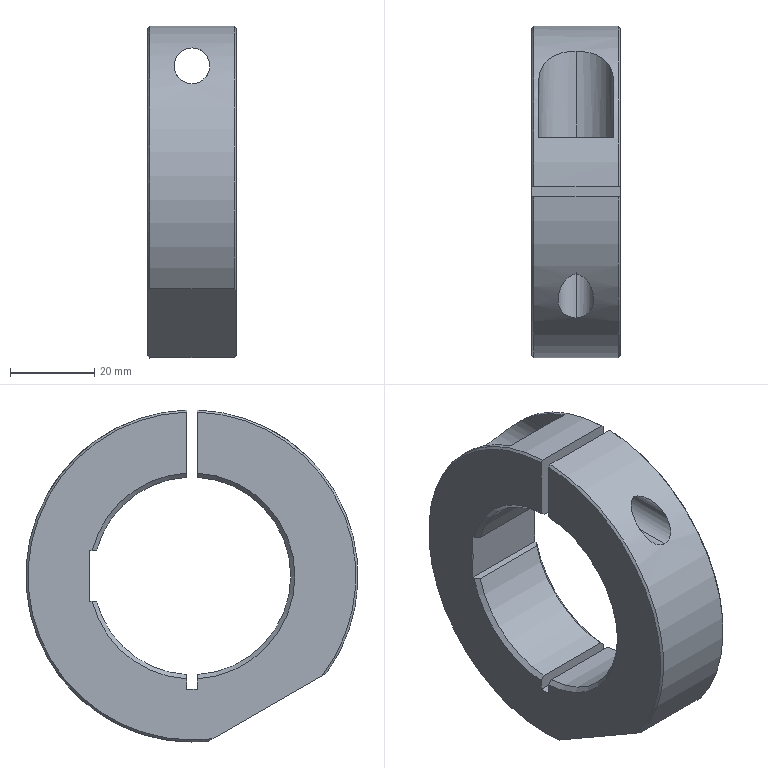Part | SolidWorks | features BaseBody 1 | 1 solid | 38 faces | box 21 x 79 x 78.98 mm | volume 57883 mm3 | plane 14 | cone 13 | cylinder 11 | commonest cylinder face diameters 47 x3 8.5 x2 11 x2 18 x2 79 x2
STEP:
#1=CARTESIAN_POINT('',(-10.5,-5.01,-38.677));
#2=VERTEX_POINT('',#1);
#3=CARTESIAN_POINT('',(-10.5,0.,-39.));
#4=VERTEX_POINT('',#3);
#5=CARTESIAN_POINT('',(-10.5,0.,0.));
#6=DIRECTION('',(1.,0.,0.));
#7=DIRECTION('',(0.,0.,-1.));
#8=AXIS2_PLACEMENT_3D('',#5,#6,#7);
#9=CIRCLE('',#8,39.);
#10=EDGE_CURVE('',#2,#4,#9,.T.);
#11=ORIENTED_EDGE('',*,*,#10,.T.);
#12=CARTESIAN_POINT('',(-10.,0.,-39.5));
#13=VERTEX_POINT('',#12);
#14=CARTESIAN_POINT('',(-10.,0.,-39.5));
#15=DIRECTION('',(0.7071,0.,-0.7071));
#16=VECTOR('',#15,1000.);
#17=LINE('',#14,#16);
#18=EDGE_CURVE('',#4,#13,#17,.T.);
#19=ORIENTED_EDGE('',*,*,#18,.T.);
#20=CARTESIAN_POINT('',(-10.,-3.922,-39.305));
#21=VERTEX_POINT('',#20);
#22=CARTESIAN_POINT('',(-10.,0.,0.));
#23=DIRECTION('',(-1.,0.,0.));
#24=DIRECTION('',(0.,0.,-1.));
#25=AXIS2_PLACEMENT_3D('',#22,#23,#24);
#26=CIRCLE('',#25,39.5);
#27=EDGE_CURVE('',#13,#21,#26,.T.);
#28=ORIENTED_EDGE('',*,*,#27,.T.);
#29=CARTESIAN_POINT('',(-10.,-3.922,-39.305));
#30=CARTESIAN_POINT('',(-10.173,-4.286,-39.095));
#31=CARTESIAN_POINT('',(-10.34,-4.648,-38.886));
#32=CARTESIAN_POINT('',(-10.5,-5.01,-38.677));
#33=B_SPLINE_CURVE_WITH_KNOTS('',3,(#29,#30,#31,#32),.UNSPECIFIED.,.F.,.F.,(4,4),(0.,1.),.UNSPECIFIED.);
#34=EDGE_CURVE('',#21,#2,#33,.T.);
#35=ORIENTED_EDGE('',*,*,#34,.T.);
#36=EDGE_LOOP('',(#11,#19,#28,#35));
#37=FACE_OUTER_BOUND('',#36,.T.);
#38=CARTESIAN_POINT('',(-10.,0.,0.));
#39=DIRECTION('',(1.,0.,0.));
#40=DIRECTION('',(0.,0.,-1.));
#41=AXIS2_PLACEMENT_3D('',#38,#39,#40);
#42=CONICAL_SURFACE('',#41,39.5,0.7854);
#43=ADVANCED_FACE('',(#37),#42,.T.);
#44=CARTESIAN_POINT('',(0.,1.25,35.5));
#45=VERTEX_POINT('',#44);
#46=CARTESIAN_POINT('',(0.,1.25,24.5));
#47=VERTEX_POINT('',#46);
#48=CARTESIAN_POINT('',(0.,1.25,30.));
#49=DIRECTION('',(0.,-1.,0.));
#50=DIRECTION('',(0.,0.,1.));
#51=AXIS2_PLACEMENT_3D('',#48,#49,#50);
#52=CIRCLE('',#51,5.5);
#53=EDGE_CURVE('',#45,#47,#52,.T.);
#54=ORIENTED_EDGE('',*,*,#53,.T.);
#55=CARTESIAN_POINT('',(0.,13.,24.5));
#56=VERTEX_POINT('',#55);
#57=CARTESIAN_POINT('',(0.,-14.306,24.5));
#58=DIRECTION('',(0.,1.,0.));
#59=VECTOR('',#58,1000.);
#60=LINE('',#57,#59);
#61=EDGE_CURVE('',#47,#56,#60,.T.);
#62=ORIENTED_EDGE('',*,*,#61,.T.);
#63=CARTESIAN_POINT('',(0.,13.,35.5));
#64=VERTEX_POINT('',#63);
#65=CARTESIAN_POINT('',(0.,13.,30.));
#66=DIRECTION('',(0.,-1.,0.));
#67=DIRECTION('',(0.,0.,1.));
#68=AXIS2_PLACEMENT_3D('',#65,#66,#67);
#69=CIRCLE('',#68,5.5);
#70=EDGE_CURVE('',#64,#56,#69,.T.);
#71=ORIENTED_EDGE('',*,*,#70,.F.);
#72=CARTESIAN_POINT('',(0.,-14.306,35.5));
#73=DIRECTION('',(0.,1.,0.));
#74=VECTOR('',#73,1000.);
#75=LINE('',#72,#74);
#76=EDGE_CURVE('',#45,#64,#75,.T.);
#77=ORIENTED_EDGE('',*,*,#76,.F.);
#78=EDGE_LOOP('',(#54,#62,#71,#77));
#79=FACE_OUTER_BOUND('',#78,.T.);
#80=CARTESIAN_POINT('',(0.,-14.306,30.));
#81=DIRECTION('',(0.,1.,0.));
#82=DIRECTION('',(0.,0.,1.));
#83=AXIS2_PLACEMENT_3D('',#80,#81,#82);
#84=CYLINDRICAL_SURFACE('',#83,5.5);
#85=ADVANCED_FACE('',(#79),#84,.F.);
#86=CARTESIAN_POINT('',(0.,-29.953,25.75));
#87=VERTEX_POINT('',#86);
#88=CARTESIAN_POINT('',(0.,-19.677,34.25));
#89=VERTEX_POINT('',#88);
#90=CARTESIAN_POINT('',(0.,-29.953,25.75));
#91=CARTESIAN_POINT('',(-0.3676,-29.953,25.75));
#92=CARTESIAN_POINT('',(-0.7239,-29.913,25.797));
#93=CARTESIAN_POINT('',(-1.243,-29.796,25.932));
#94=CARTESIAN_POINT('',(-1.411,-29.748,25.987));
#95=CARTESIAN_POINT('',(-1.731,-29.636,26.115));
#96=CARTESIAN_POINT('',(-1.885,-29.572,26.187));
#97=CARTESIAN_POINT('',(-2.18,-29.429,26.348));
#98=CARTESIAN_POINT('',(-2.321,-29.35,26.436));
#99=CARTESIAN_POINT('',(-2.583,-29.182,26.621));
#100=CARTESIAN_POINT('',(-2.706,-29.092,26.719));
#101=CARTESIAN_POINT('',(-3.052,-28.809,27.026));
#102=CARTESIAN_POINT('',(-3.253,-28.597,27.25));
#103=CARTESIAN_POINT('',(-3.592,-28.152,27.71));
#104=CARTESIAN_POINT('',(-3.73,-27.917,27.946));
#105=CARTESIAN_POINT('',(-3.957,-27.427,28.428));
#106=CARTESIAN_POINT('',(-4.046,-27.17,28.674));
#107=CARTESIAN_POINT('',(-4.237,-26.389,29.4));
#108=CARTESIAN_POINT('',(-4.274,-25.85,29.875));
#109=CARTESIAN_POINT('',(-4.218,-25.015,30.572));
#110=CARTESIAN_POINT('',(-4.18,-24.734,30.799));
#111=CARTESIAN_POINT('',(-4.071,-24.174,31.241));
#112=CARTESIAN_POINT('',(-4.,-23.894,31.455));
#113=CARTESIAN_POINT('',(-3.733,-23.054,32.082));
#114=CARTESIAN_POINT('',(-3.486,-22.49,32.479));
#115=CARTESIAN_POINT('',(-3.003,-21.685,33.017));
#116=CARTESIAN_POINT('',(-2.823,-21.422,33.188));
#117=CARTESIAN_POINT('',(-2.411,-20.915,33.51));
#118=CARTESIAN_POINT('',(-2.182,-20.674,33.659));
#119=CARTESIAN_POINT('',(-1.793,-20.348,33.856));
#120=CARTESIAN_POINT('',(-1.654,-20.245,33.918));
#121=CARTESIAN_POINT('',(-1.363,-20.058,34.029));
#122=CARTESIAN_POINT('',(-1.21,-19.974,34.078));
#123=CARTESIAN_POINT('',(-0.8856,-19.833,34.16));
#124=CARTESIAN_POINT('',(-0.713,-19.775,34.193));
#125=CARTESIAN_POINT('',(-0.3632,-19.698,34.238));
#126=CARTESIAN_POINT('',(-0.1844,-19.677,34.25));
#127=CARTESIAN_POINT('',(0.,-19.677,34.25));
#128=B_SPLINE_CURVE_WITH_KNOTS('',3,(#90,#91,#92,#93,#94,#95,#96,#97,#98,#99,#100,#101,#102,#103,#104,#105,#106,#107,#108,#109,#110,#111,#112,#113,#114,#115,#116,#117,#118,#119,#120,#121,#122,#123,#124,#125,#126,#127),.UNSPECIFIED.,.F.,.F.,(4,2,2,2,2,2,2,2,2,2,2,2,2,2,2,2,2,2,4),(0.01741,0.0185,0.01905,0.01959,0.02014,0.02068,0.02177,0.02286,0.02395,0.02613,0.02721,0.0283,0.03048,0.03157,0.03266,0.0332,0.03375,0.03429,0.03484),.UNSPECIFIED.);
#129=EDGE_CURVE('',#87,#89,#128,.T.);
#130=ORIENTED_EDGE('',*,*,#129,.F.);
#131=CARTESIAN_POINT('',(0.,-1.25,25.75));
#132=VERTEX_POINT('',#131);
#133=CARTESIAN_POINT('',(0.,-1.25,25.75));
#134=DIRECTION('',(0.,1.,0.));
#135=VECTOR('',#134,1000.);
#136=LINE('',#133,#135);
#137=EDGE_CURVE('',#87,#132,#136,.T.);
#138=ORIENTED_EDGE('',*,*,#137,.T.);
#139=CARTESIAN_POINT('',(0.,-1.25,34.25));
#140=VERTEX_POINT('',#139);
#141=CARTESIAN_POINT('',(0.,-1.25,30.));
#142=DIRECTION('',(0.,1.,0.));
#143=DIRECTION('',(0.,0.,1.));
#144=AXIS2_PLACEMENT_3D('',#141,#142,#143);
#145=CIRCLE('',#144,4.25);
#146=EDGE_CURVE('',#132,#140,#145,.T.);
#147=ORIENTED_EDGE('',*,*,#146,.T.);
#148=CARTESIAN_POINT('',(0.,-1.25,34.25));
#149=DIRECTION('',(0.,1.,0.));
#150=VECTOR('',#149,1000.);
#151=LINE('',#148,#150);
#152=EDGE_CURVE('',#89,#140,#151,.T.);
#153=ORIENTED_EDGE('',*,*,#152,.F.);
#154=EDGE_LOOP('',(#130,#138,#147,#153));
#155=FACE_OUTER_BOUND('',#154,.T.);
#156=CARTESIAN_POINT('',(0.,-1.25,30.));
#157=DIRECTION('',(0.,1.,0.));
#158=DIRECTION('',(0.,0.,1.));
#159=AXIS2_PLACEMENT_3D('',#156,#157,#158);
#160=CYLINDRICAL_SURFACE('',#159,4.25);
#161=ADVANCED_FACE('',(#155),#160,.F.);
#162=CARTESIAN_POINT('',(0.,33.455,21.));
#163=VERTEX_POINT('',#162);
#164=CARTESIAN_POINT('',(9.,25.695,30.));
#165=VERTEX_POINT('',#164);
#166=CARTESIAN_POINT('',(0.,33.455,21.));
#167=CARTESIAN_POINT('',(0.7019,33.455,21.));
#168=CARTESIAN_POINT('',(1.387,33.405,21.081));
#169=CARTESIAN_POINT('',(2.391,33.254,21.317));
#170=CARTESIAN_POINT('',(2.724,33.191,21.415));
#171=CARTESIAN_POINT('',(3.363,33.042,21.645));
#172=CARTESIAN_POINT('',(3.672,32.956,21.776));
#173=CARTESIAN_POINT('',(4.268,32.76,22.07));
#174=CARTESIAN_POINT('',(4.556,32.651,22.231));
#175=CARTESIAN_POINT('',(5.109,32.408,22.584));
#176=CARTESIAN_POINT('',(5.372,32.276,22.772));
#177=CARTESIAN_POINT('',(5.867,31.993,23.168));
#178=CARTESIAN_POINT('',(6.1,31.842,23.375));
#179=CARTESIAN_POINT('',(6.538,31.52,23.807));
#180=CARTESIAN_POINT('',(6.745,31.349,24.033));
#181=CARTESIAN_POINT('',(7.316,30.81,24.725));
#182=CARTESIAN_POINT('',(7.635,30.422,25.203));
#183=CARTESIAN_POINT('',(8.034,29.796,25.934));
#184=CARTESIAN_POINT('',(8.154,29.578,26.182));
#185=CARTESIAN_POINT('',(8.367,29.135,26.674));
#186=CARTESIAN_POINT('',(8.46,28.908,26.92));
#187=CARTESIAN_POINT('',(8.703,28.216,27.651));
#188=CARTESIAN_POINT('',(8.817,27.736,28.132));
#189=CARTESIAN_POINT('',(8.966,26.742,29.079));
#190=CARTESIAN_POINT('',(9.,26.225,29.547));
#191=CARTESIAN_POINT('',(9.,25.695,30.));
#192=B_SPLINE_CURVE_WITH_KNOTS('',3,(#166,#167,#168,#169,#170,#171,#172,#173,#174,#175,#176,#177,#178,#179,#180,#181,#182,#183,#184,#185,#186,#187,#188,#189,#190,#191),.UNSPECIFIED.,.F.,.F.,(4,2,2,2,2,2,2,2,2,2,2,2,4),(0.,0.002074,0.003111,0.004148,0.005185,0.006222,0.00726,0.008297,0.01037,0.01141,0.01244,0.01452,0.01659),.UNSPECIFIED.);
#193=EDGE_CURVE('',#163,#165,#192,.T.);
#194=ORIENTED_EDGE('',*,*,#193,.F.);
#195=CARTESIAN_POINT('',(0.,13.,21.));
#196=VERTEX_POINT('',#195);
#197=CARTESIAN_POINT('',(0.,39.5,21.));
#198=DIRECTION('',(0.,-1.,0.));
#199=VECTOR('',#198,1000.);
#200=LINE('',#197,#199);
#201=EDGE_CURVE('',#163,#196,#200,.T.);
#202=ORIENTED_EDGE('',*,*,#201,.T.);
#203=CARTESIAN_POINT('',(9.,13.,30.));
#204=VERTEX_POINT('',#203);
#205=CARTESIAN_POINT('',(0.,13.,30.));
#206=DIRECTION('',(0.,-1.,0.));
#207=DIRECTION('',(0.,0.,-1.));
#208=AXIS2_PLACEMENT_3D('',#205,#206,#207);
#209=CIRCLE('',#208,9.);
#210=EDGE_CURVE('',#196,#204,#209,.T.);
#211=ORIENTED_EDGE('',*,*,#210,.T.);
#212=CARTESIAN_POINT('',(9.,39.5,30.));
#213=DIRECTION('',(0.,-1.,0.));
#214=VECTOR('',#213,1000.);
#215=LINE('',#212,#214);
#216=EDGE_CURVE('',#165,#204,#215,.T.);
#217=ORIENTED_EDGE('',*,*,#216,.F.);
#218=EDGE_LOOP('',(#194,#202,#211,#217));
#219=FACE_OUTER_BOUND('',#218,.T.);
#220=CARTESIAN_POINT('',(0.,39.5,30.));
#221=DIRECTION('',(0.,-1.,0.));
#222=DIRECTION('',(0.,0.,-1.));
#223=AXIS2_PLACEMENT_3D('',#220,#221,#222);
#224=CYLINDRICAL_SURFACE('',#223,9.);
#225=ADVANCED_FACE('',(#219),#224,.F.);
#226=CARTESIAN_POINT('',(-10.5,24.3,3.124));
#227=VERTEX_POINT('',#226);
#228=CARTESIAN_POINT('',(-10.5,24.3,-3.124));
#229=VERTEX_POINT('',#228);
#230=CARTESIAN_POINT('',(-10.5,0.,0.));
#231=DIRECTION('',(-1.,0.,0.));
#232=DIRECTION('',(0.,0.,1.));
#233=AXIS2_PLACEMENT_3D('',#230,#231,#232);
#234=CIRCLE('',#233,24.5);
#235=EDGE_CURVE('',#227,#229,#234,.T.);
#236=ORIENTED_EDGE('',*,*,#235,.F.);
#237=CARTESIAN_POINT('',(-10.5,24.3,6.));
#238=VERTEX_POINT('',#237);
#239=CARTESIAN_POINT('',(-10.5,24.3,0.));
#240=DIRECTION('',(0.,0.,-1.));
#241=VECTOR('',#240,1000.);
#242=LINE('',#239,#241);
#243=EDGE_CURVE('',#238,#227,#242,.T.);
#244=ORIENTED_EDGE('',*,*,#243,.F.);
#245=CARTESIAN_POINT('',(-10.5,23.754,6.));
#246=VERTEX_POINT('',#245);
#247=CARTESIAN_POINT('',(-10.5,24.3,6.));
#248=DIRECTION('',(0.,-1.,0.));
#249=VECTOR('',#248,1000.);
#250=LINE('',#247,#249);
#251=EDGE_CURVE('',#238,#246,#250,.T.);
#252=ORIENTED_EDGE('',*,*,#251,.T.);
#253=CARTESIAN_POINT('',(-10.5,1.25,24.468));
#254=VERTEX_POINT('',#253);
#255=CARTESIAN_POINT('',(-10.5,0.,0.));
#256=DIRECTION('',(-1.,0.,0.));
#257=DIRECTION('',(0.,0.,1.));
#258=AXIS2_PLACEMENT_3D('',#255,#256,#257);
#259=CIRCLE('',#258,24.5);
#260=EDGE_CURVE('',#254,#246,#259,.T.);
#261=ORIENTED_EDGE('',*,*,#260,.F.);
#262=CARTESIAN_POINT('',(-10.5,1.25,38.98));
#263=VERTEX_POINT('',#262);
#264=CARTESIAN_POINT('',(-10.5,1.25,0.));
#265=DIRECTION('',(0.,0.,-1.));
#266=VECTOR('',#265,1000.);
#267=LINE('',#264,#266);
#268=EDGE_CURVE('',#263,#254,#267,.T.);
#269=ORIENTED_EDGE('',*,*,#268,.F.);
#270=CARTESIAN_POINT('',(-10.5,0.,0.));
#271=DIRECTION('',(1.,0.,0.));
#272=DIRECTION('',(0.,0.,-1.));
#273=AXIS2_PLACEMENT_3D('',#270,#271,#272);
#274=CIRCLE('',#273,39.);
#275=EDGE_CURVE('',#4,#263,#274,.T.);
#276=ORIENTED_EDGE('',*,*,#275,.F.);
#277=ORIENTED_EDGE('',*,*,#10,.F.);
#278=CARTESIAN_POINT('',(-10.5,-30.99,-23.677));
#279=VERTEX_POINT('',#278);
#280=CARTESIAN_POINT('',(-10.5,-30.99,-23.677));
#281=DIRECTION('',(0.,0.866,-0.5));
#282=VECTOR('',#281,1000.);
#283=LINE('',#280,#282);
#284=EDGE_CURVE('',#279,#2,#283,.T.);
#285=ORIENTED_EDGE('',*,*,#284,.F.);
#286=CARTESIAN_POINT('',(-10.5,-1.25,38.98));
#287=VERTEX_POINT('',#286);
#288=CARTESIAN_POINT('',(-10.5,0.,0.));
#289=DIRECTION('',(1.,0.,0.));
#290=DIRECTION('',(0.,0.,-1.));
#291=AXIS2_PLACEMENT_3D('',#288,#289,#290);
#292=CIRCLE('',#291,39.);
#293=EDGE_CURVE('',#287,#279,#292,.T.);
#294=ORIENTED_EDGE('',*,*,#293,.F.);
#295=CARTESIAN_POINT('',(-10.5,-1.25,24.468));
#296=VERTEX_POINT('',#295);
#297=CARTESIAN_POINT('',(-10.5,-1.25,0.));
#298=DIRECTION('',(0.,0.,1.));
#299=VECTOR('',#298,1000.);
#300=LINE('',#297,#299);
#301=EDGE_CURVE('',#296,#287,#300,.T.);
#302=ORIENTED_EDGE('',*,*,#301,.F.);
#303=CARTESIAN_POINT('',(-10.5,-1.25,-24.468));
#304=VERTEX_POINT('',#303);
#305=CARTESIAN_POINT('',(-10.5,0.,0.));
#306=DIRECTION('',(-1.,0.,0.));
#307=DIRECTION('',(0.,0.,1.));
#308=AXIS2_PLACEMENT_3D('',#305,#306,#307);
#309=CIRCLE('',#308,24.5);
#310=EDGE_CURVE('',#304,#296,#309,.T.);
#311=ORIENTED_EDGE('',*,*,#310,.F.);
#312=CARTESIAN_POINT('',(-10.5,-1.25,-27.));
#313=VERTEX_POINT('',#312);
#314=CARTESIAN_POINT('',(-10.5,-1.25,0.));
#315=DIRECTION('',(0.,0.,1.));
#316=VECTOR('',#315,1000.);
#317=LINE('',#314,#316);
#318=EDGE_CURVE('',#313,#304,#317,.T.);
#319=ORIENTED_EDGE('',*,*,#318,.F.);
#320=CARTESIAN_POINT('',(-10.5,1.25,-27.));
#321=VERTEX_POINT('',#320);
#322=CARTESIAN_POINT('',(-10.5,0.,-27.));
#323=DIRECTION('',(0.,-1.,0.));
#324=VECTOR('',#323,1000.);
#325=LINE('',#322,#324);
#326=EDGE_CURVE('',#321,#313,#325,.T.);
#327=ORIENTED_EDGE('',*,*,#326,.F.);
#328=CARTESIAN_POINT('',(-10.5,1.25,-24.468));
#329=VERTEX_POINT('',#328);
#330=CARTESIAN_POINT('',(-10.5,1.25,0.));
#331=DIRECTION('',(0.,0.,-1.));
#332=VECTOR('',#331,1000.);
#333=LINE('',#330,#332);
#334=EDGE_CURVE('',#329,#321,#333,.T.);
#335=ORIENTED_EDGE('',*,*,#334,.F.);
#336=CARTESIAN_POINT('',(-10.5,23.754,-6.));
#337=VERTEX_POINT('',#336);
#338=CARTESIAN_POINT('',(-10.5,0.,0.));
#339=DIRECTION('',(-1.,0.,0.));
#340=DIRECTION('',(0.,0.,1.));
#341=AXIS2_PLACEMENT_3D('',#338,#339,#340);
#342=CIRCLE('',#341,24.5);
#343=EDGE_CURVE('',#337,#329,#342,.T.);
#344=ORIENTED_EDGE('',*,*,#343,.F.);
#345=CARTESIAN_POINT('',(-10.5,24.3,-6.));
#346=VERTEX_POINT('',#345);
#347=CARTESIAN_POINT('',(-10.5,20.229,-6.));
#348=DIRECTION('',(0.,1.,0.));
#349=VECTOR('',#348,1000.);
#350=LINE('',#347,#349);
#351=EDGE_CURVE('',#337,#346,#350,.T.);
#352=ORIENTED_EDGE('',*,*,#351,.T.);
#353=CARTESIAN_POINT('',(-10.5,24.3,0.));
#354=DIRECTION('',(0.,0.,-1.));
#355=VECTOR('',#354,1000.);
#356=LINE('',#353,#355);
#357=EDGE_CURVE('',#229,#346,#356,.T.);
#358=ORIENTED_EDGE('',*,*,#357,.F.);
#359=EDGE_LOOP('',(#236,#244,#252,#261,#269,#276,#277,#285,#294,#302,#311,#319,#327,#335,#344,#352,#358));
#360=FACE_OUTER_BOUND('',#359,.T.);
#361=CARTESIAN_POINT('',(-10.5,0.,0.));
#362=DIRECTION('',(1.,0.,0.));
#363=DIRECTION('',(0.,0.,-1.));
#364=AXIS2_PLACEMENT_3D('',#361,#362,#363);
#365=PLANE('',#364);
#366=ADVANCED_FACE('',(#360),#365,.F.);
#367=CARTESIAN_POINT('',(10.5,24.3,3.124));
#368=VERTEX_POINT('',#367);
#369=CARTESIAN_POINT('',(10.5,24.3,-3.124));
#370=VERTEX_POINT('',#369);
#371=CARTESIAN_POINT('',(10.5,24.3,3.124));
#372=CARTESIAN_POINT('',(10.234,24.3,1.041));
#373=CARTESIAN_POINT('',(10.234,24.3,-1.041));
#374=CARTESIAN_POINT('',(10.5,24.3,-3.124));
#375=B_SPLINE_CURVE_WITH_KNOTS('',3,(#371,#372,#373,#374),.UNSPECIFIED.,.F.,.F.,(4,4),(0.,0.006248),.UNSPECIFIED.);
#376=EDGE_CURVE('',#368,#370,#375,.T.);
#377=ORIENTED_EDGE('',*,*,#376,.F.);
#378=CARTESIAN_POINT('',(10.5,24.3,6.));
#379=VERTEX_POINT('',#378);
#380=CARTESIAN_POINT('',(10.5,24.3,-6.));
#381=DIRECTION('',(0.,0.,-1.));
#382=VECTOR('',#381,1000.);
#383=LINE('',#380,#382);
#384=EDGE_CURVE('',#379,#368,#383,.T.);
#385=ORIENTED_EDGE('',*,*,#384,.F.);
#386=CARTESIAN_POINT('',(-14.5,24.3,6.));
#387=DIRECTION('',(1.,0.,0.));
#388=VECTOR('',#387,1000.);
#389=LINE('',#386,#388);
#390=EDGE_CURVE('',#238,#379,#389,.T.);
#391=ORIENTED_EDGE('',*,*,#390,.F.);
#392=ORIENTED_EDGE('',*,*,#243,.T.);
#393=CARTESIAN_POINT('',(-10.5,24.3,-3.124));
#394=CARTESIAN_POINT('',(-10.234,24.3,-1.041));
#395=CARTESIAN_POINT('',(-10.234,24.3,1.041));
#396=CARTESIAN_POINT('',(-10.5,24.3,3.124));
#397=B_SPLINE_CURVE_WITH_KNOTS('',3,(#393,#394,#395,#396),.UNSPECIFIED.,.F.,.F.,(4,4),(0.,0.006248),.UNSPECIFIED.);
#398=EDGE_CURVE('',#229,#227,#397,.T.);
#399=ORIENTED_EDGE('',*,*,#398,.F.);
#400=ORIENTED_EDGE('',*,*,#357,.T.);
#401=CARTESIAN_POINT('',(10.5,24.3,-6.));
#402=VERTEX_POINT('',#401);
#403=CARTESIAN_POINT('',(-14.5,24.3,-6.));
#404=DIRECTION('',(-1.,0.,0.));
#405=VECTOR('',#404,1000.);
#406=LINE('',#403,#405);
#407=EDGE_CURVE('',#402,#346,#406,.T.);
#408=ORIENTED_EDGE('',*,*,#407,.F.);
#409=CARTESIAN_POINT('',(10.5,24.3,-6.));
#410=DIRECTION('',(0.,0.,-1.));
#411=VECTOR('',#410,1000.);
#412=LINE('',#409,#411);
#413=EDGE_CURVE('',#370,#402,#412,.T.);
#414=ORIENTED_EDGE('',*,*,#413,.F.);
#415=EDGE_LOOP('',(#377,#385,#391,#392,#399,#400,#408,#414));
#416=FACE_OUTER_BOUND('',#415,.T.);
#417=CARTESIAN_POINT('',(-14.5,24.3,-6.));
#418=DIRECTION('',(0.,1.,0.));
#419=DIRECTION('',(0.,0.,1.));
#420=AXIS2_PLACEMENT_3D('',#417,#418,#419);
#421=PLANE('',#420);
#422=ADVANCED_FACE('',(#416),#421,.F.);
#423=ORIENTED_EDGE('',*,*,#398,.T.);
#424=ORIENTED_EDGE('',*,*,#235,.T.);
#425=EDGE_LOOP('',(#423,#424));
#426=FACE_OUTER_BOUND('',#425,.T.);
#427=CARTESIAN_POINT('',(-10.5,0.,0.));
#428=DIRECTION('',(-1.,0.,0.));
#429=DIRECTION('',(0.,0.,1.));
#430=AXIS2_PLACEMENT_3D('',#427,#428,#429);
#431=CONICAL_SURFACE('',#430,24.5,0.7854);
#432=ADVANCED_FACE('',(#426),#431,.F.);
#433=CARTESIAN_POINT('',(-9.5,1.25,23.467));
#434=VERTEX_POINT('',#433);
#435=CARTESIAN_POINT('',(-10.5,1.25,24.468));
#436=CARTESIAN_POINT('',(-10.167,1.25,24.134));
#437=CARTESIAN_POINT('',(-9.833,1.25,23.801));
#438=CARTESIAN_POINT('',(-9.5,1.25,23.467));
#439=B_SPLINE_CURVE_WITH_KNOTS('',3,(#435,#436,#437,#438),.UNSPECIFIED.,.F.,.F.,(4,4),(0.,0.001415),.UNSPECIFIED.);
#440=EDGE_CURVE('',#254,#434,#439,.T.);
#441=ORIENTED_EDGE('',*,*,#440,.F.);
#442=ORIENTED_EDGE('',*,*,#260,.T.);
#443=CARTESIAN_POINT('',(-9.5,22.721,6.));
#444=VERTEX_POINT('',#443);
#445=CARTESIAN_POINT('',(-9.5,22.721,6.));
#446=CARTESIAN_POINT('',(-9.833,23.066,6.));
#447=CARTESIAN_POINT('',(-10.166,23.41,6.));
#448=CARTESIAN_POINT('',(-10.5,23.754,6.));
#449=B_SPLINE_CURVE_WITH_KNOTS('',3,(#445,#446,#447,#448),.UNSPECIFIED.,.F.,.F.,(4,4),(0.,0.001438),.UNSPECIFIED.);
#450=EDGE_CURVE('',#444,#246,#449,.T.);
#451=ORIENTED_EDGE('',*,*,#450,.F.);
#452=CARTESIAN_POINT('',(-9.5,0.,0.));
#453=DIRECTION('',(-1.,0.,0.));
#454=DIRECTION('',(0.,0.,1.));
#455=AXIS2_PLACEMENT_3D('',#452,#453,#454);
#456=CIRCLE('',#455,23.5);
#457=EDGE_CURVE('',#434,#444,#456,.T.);
#458=ORIENTED_EDGE('',*,*,#457,.F.);
#459=EDGE_LOOP('',(#441,#442,#451,#458));
#460=FACE_OUTER_BOUND('',#459,.T.);
#461=CARTESIAN_POINT('',(-10.5,0.,0.));
#462=DIRECTION('',(-1.,0.,0.));
#463=DIRECTION('',(0.,0.,1.));
#464=AXIS2_PLACEMENT_3D('',#461,#462,#463);
#465=CONICAL_SURFACE('',#464,24.5,0.7854);
#466=ADVANCED_FACE('',(#460),#465,.F.);
#467=ORIENTED_EDGE('',*,*,#53,.F.);
#468=CARTESIAN_POINT('',(0.,1.25,30.));
#469=DIRECTION('',(0.,-1.,0.));
#470=DIRECTION('',(0.,0.,1.));
#471=AXIS2_PLACEMENT_3D('',#468,#469,#470);
#472=CIRCLE('',#471,5.5);
#473=EDGE_CURVE('',#47,#45,#472,.T.);
#474=ORIENTED_EDGE('',*,*,#473,.F.);
#475=EDGE_LOOP('',(#467,#474));
#476=FACE_BOUND('',#475,.T.);
#477=CARTESIAN_POINT('',(9.5,1.25,23.467));
#478=VERTEX_POINT('',#477);
#479=CARTESIAN_POINT('',(10.5,1.25,24.468));
#480=VERTEX_POINT('',#479);
#481=CARTESIAN_POINT('',(9.5,1.25,23.467));
#482=CARTESIAN_POINT('',(9.833,1.25,23.801));
#483=CARTESIAN_POINT('',(10.167,1.25,24.134));
#484=CARTESIAN_POINT('',(10.5,1.25,24.468));
#485=B_SPLINE_CURVE_WITH_KNOTS('',3,(#481,#482,#483,#484),.UNSPECIFIED.,.F.,.F.,(4,4),(0.,0.001415),.UNSPECIFIED.);
#486=EDGE_CURVE('',#478,#480,#485,.T.);
#487=ORIENTED_EDGE('',*,*,#486,.T.);
#488=CARTESIAN_POINT('',(10.5,1.25,38.98));
#489=VERTEX_POINT('',#488);
#490=CARTESIAN_POINT('',(10.5,1.25,53.848));
#491=DIRECTION('',(0.,0.,-1.));
#492=VECTOR('',#491,1000.);
#493=LINE('',#490,#492);
#494=EDGE_CURVE('',#489,#480,#493,.T.);
#495=ORIENTED_EDGE('',*,*,#494,.F.);
#496=CARTESIAN_POINT('',(10.,1.25,39.48));
#497=VERTEX_POINT('',#496);
#498=CARTESIAN_POINT('',(10.,1.25,39.48));
#499=CARTESIAN_POINT('',(10.167,1.25,39.313));
#500=CARTESIAN_POINT('',(10.333,1.25,39.147));
#501=CARTESIAN_POINT('',(10.5,1.25,38.98));
#502=B_SPLINE_CURVE_WITH_KNOTS('',3,(#498,#499,#500,#501),.UNSPECIFIED.,.F.,.F.,(4,4),(0.,0.0007073),.UNSPECIFIED.);
#503=EDGE_CURVE('',#497,#489,#502,.T.);
#504=ORIENTED_EDGE('',*,*,#503,.F.);
#505=CARTESIAN_POINT('',(-10.,1.25,39.48));
#506=VERTEX_POINT('',#505);
#507=CARTESIAN_POINT('',(-10.5,1.25,39.48));
#508=DIRECTION('',(1.,0.,0.));
#509=VECTOR('',#508,1000.);
#510=LINE('',#507,#509);
#511=EDGE_CURVE('',#506,#497,#510,.T.);
#512=ORIENTED_EDGE('',*,*,#511,.F.);
#513=CARTESIAN_POINT('',(-10.5,1.25,38.98));
#514=CARTESIAN_POINT('',(-10.333,1.25,39.147));
#515=CARTESIAN_POINT('',(-10.167,1.25,39.313));
#516=CARTESIAN_POINT('',(-10.,1.25,39.48));
#517=B_SPLINE_CURVE_WITH_KNOTS('',3,(#513,#514,#515,#516),.UNSPECIFIED.,.F.,.F.,(4,4),(0.,0.0007073),.UNSPECIFIED.);
#518=EDGE_CURVE('',#263,#506,#517,.T.);
#519=ORIENTED_EDGE('',*,*,#518,.F.);
#520=ORIENTED_EDGE('',*,*,#268,.T.);
#521=ORIENTED_EDGE('',*,*,#440,.T.);
#522=CARTESIAN_POINT('',(-10.5,1.25,23.467));
#523=DIRECTION('',(-1.,0.,0.));
#524=VECTOR('',#523,1000.);
#525=LINE('',#522,#524);
#526=EDGE_CURVE('',#478,#434,#525,.T.);
#527=ORIENTED_EDGE('',*,*,#526,.F.);
#528=EDGE_LOOP('',(#487,#495,#504,#512,#519,#520,#521,#527));
#529=FACE_OUTER_BOUND('',#528,.T.);
#530=CARTESIAN_POINT('',(-10.5,1.25,53.848));
#531=DIRECTION('',(0.,1.,0.));
#532=DIRECTION('',(0.,0.,1.));
#533=AXIS2_PLACEMENT_3D('',#530,#531,#532);
#534=PLANE('',#533);
#535=ADVANCED_FACE('',(#476,#529),#534,.F.);
#536=ORIENTED_EDGE('',*,*,#18,.F.);
#537=ORIENTED_EDGE('',*,*,#275,.T.);
#538=ORIENTED_EDGE('',*,*,#518,.T.);
#539=CARTESIAN_POINT('',(-10.,0.,0.));
#540=DIRECTION('',(-1.,0.,0.));
#541=DIRECTION('',(0.,0.,-1.));
#542=AXIS2_PLACEMENT_3D('',#539,#540,#541);
#543=CIRCLE('',#542,39.5);
#544=EDGE_CURVE('',#506,#13,#543,.T.);
#545=ORIENTED_EDGE('',*,*,#544,.T.);
#546=EDGE_LOOP('',(#536,#537,#538,#545));
#547=FACE_OUTER_BOUND('',#546,.T.);
#548=CARTESIAN_POINT('',(-10.,0.,0.));
#549=DIRECTION('',(1.,0.,0.));
#550=DIRECTION('',(0.,0.,-1.));
#551=AXIS2_PLACEMENT_3D('',#548,#549,#550);
#552=CONICAL_SURFACE('',#551,39.5,0.7854);
#553=ADVANCED_FACE('',(#547),#552,.T.);
#554=CARTESIAN_POINT('',(10.5,-5.01,-38.677));
#555=VERTEX_POINT('',#554);
#556=CARTESIAN_POINT('',(10.,-3.922,-39.305));
#557=VERTEX_POINT('',#556);
#558=CARTESIAN_POINT('',(10.5,-5.01,-38.677));
#559=CARTESIAN_POINT('',(10.34,-4.648,-38.886));
#560=CARTESIAN_POINT('',(10.173,-4.286,-39.095));
#561=CARTESIAN_POINT('',(10.,-3.922,-39.305));
#562=B_SPLINE_CURVE_WITH_KNOTS('',3,(#558,#559,#560,#561),.UNSPECIFIED.,.F.,.F.,(4,4),(0.,1.),.UNSPECIFIED.);
#563=EDGE_CURVE('',#555,#557,#562,.T.);
#564=ORIENTED_EDGE('',*,*,#563,.F.);
#565=CARTESIAN_POINT('',(10.5,-30.99,-23.677));
#566=VERTEX_POINT('',#565);
#567=CARTESIAN_POINT('',(10.5,11.116,-47.987));
#568=DIRECTION('',(0.,0.866,-0.5));
#569=VECTOR('',#568,1000.);
#570=LINE('',#567,#569);
#571=EDGE_CURVE('',#566,#555,#570,.T.);
#572=ORIENTED_EDGE('',*,*,#571,.F.);
#573=CARTESIAN_POINT('',(10.,-32.078,-23.049));
#574=VERTEX_POINT('',#573);
#575=CARTESIAN_POINT('',(10.,-32.078,-23.049));
#576=CARTESIAN_POINT('',(10.173,-31.714,-23.259));
#577=CARTESIAN_POINT('',(10.34,-31.352,-23.468));
#578=CARTESIAN_POINT('',(10.5,-30.99,-23.677));
#579=B_SPLINE_CURVE_WITH_KNOTS('',3,(#575,#576,#577,#578),.UNSPECIFIED.,.F.,.F.,(4,4),(0.,1.),.UNSPECIFIED.);
#580=EDGE_CURVE('',#574,#566,#579,.T.);
#581=ORIENTED_EDGE('',*,*,#580,.F.);
#582=CARTESIAN_POINT('',(-10.,-32.078,-23.049));
#583=VERTEX_POINT('',#582);
#584=CARTESIAN_POINT('',(-10.5,-32.078,-23.049));
#585=DIRECTION('',(1.,0.,0.));
#586=VECTOR('',#585,1000.);
#587=LINE('',#584,#586);
#588=EDGE_CURVE('',#583,#574,#587,.T.);
#589=ORIENTED_EDGE('',*,*,#588,.F.);
#590=CARTESIAN_POINT('',(-10.5,-30.99,-23.677));
#591=CARTESIAN_POINT('',(-10.34,-31.352,-23.468));
#592=CARTESIAN_POINT('',(-10.173,-31.714,-23.259));
#593=CARTESIAN_POINT('',(-10.,-32.078,-23.049));
#594=B_SPLINE_CURVE_WITH_KNOTS('',3,(#590,#591,#592,#593),.UNSPECIFIED.,.F.,.F.,(4,4),(0.,1.),.UNSPECIFIED.);
#595=EDGE_CURVE('',#279,#583,#594,.T.);
#596=ORIENTED_EDGE('',*,*,#595,.F.);
#597=ORIENTED_EDGE('',*,*,#284,.T.);
#598=ORIENTED_EDGE('',*,*,#34,.F.);
#599=CARTESIAN_POINT('',(-10.5,-3.922,-39.305));
#600=DIRECTION('',(-1.,0.,0.));
#601=VECTOR('',#600,1000.);
#602=LINE('',#599,#601);
#603=EDGE_CURVE('',#557,#21,#602,.T.);
#604=ORIENTED_EDGE('',*,*,#603,.F.);
#605=EDGE_LOOP('',(#564,#572,#581,#589,#596,#597,#598,#604));
#606=FACE_OUTER_BOUND('',#605,.T.);
#607=CARTESIAN_POINT('',(-10.5,11.116,-47.987));
#608=DIRECTION('',(0.,0.5,0.866));
#609=DIRECTION('',(0.,-0.866,0.5));
#610=AXIS2_PLACEMENT_3D('',#607,#608,#609);
#611=PLANE('',#610);
#612=ADVANCED_FACE('',(#606),#611,.F.);
#613=CARTESIAN_POINT('',(-10.,-1.25,39.48));
#614=VERTEX_POINT('',#613);
#615=CARTESIAN_POINT('',(-10.,0.,0.));
#616=DIRECTION('',(-1.,0.,0.));
#617=DIRECTION('',(0.,0.,-1.));
#618=AXIS2_PLACEMENT_3D('',#615,#616,#617);
#619=CIRCLE('',#618,39.5);
#620=EDGE_CURVE('',#583,#614,#619,.T.);
#621=ORIENTED_EDGE('',*,*,#620,.T.);
#622=CARTESIAN_POINT('',(-10.,-1.25,39.48));
#623=CARTESIAN_POINT('',(-10.167,-1.25,39.313));
#624=CARTESIAN_POINT('',(-10.333,-1.25,39.147));
#625=CARTESIAN_POINT('',(-10.5,-1.25,38.98));
#626=B_SPLINE_CURVE_WITH_KNOTS('',3,(#622,#623,#624,#625),.UNSPECIFIED.,.F.,.F.,(4,4),(0.,0.0007073),.UNSPECIFIED.);
#627=EDGE_CURVE('',#614,#287,#626,.T.);
#628=ORIENTED_EDGE('',*,*,#627,.T.);
#629=ORIENTED_EDGE('',*,*,#293,.T.);
#630=ORIENTED_EDGE('',*,*,#595,.T.);
#631=EDGE_LOOP('',(#621,#628,#629,#630));
#632=FACE_OUTER_BOUND('',#631,.T.);
#633=CARTESIAN_POINT('',(-10.,0.,0.));
#634=DIRECTION('',(1.,0.,0.));
#635=DIRECTION('',(0.,0.,-1.));
#636=AXIS2_PLACEMENT_3D('',#633,#634,#635);
#637=CONICAL_SURFACE('',#636,39.5,0.7854);
#638=ADVANCED_FACE('',(#632),#637,.T.);
#639=CARTESIAN_POINT('',(0.,-1.25,30.));
#640=DIRECTION('',(0.,1.,0.));
#641=DIRECTION('',(0.,0.,1.));
#642=AXIS2_PLACEMENT_3D('',#639,#640,#641);
#643=CIRCLE('',#642,4.25);
#644=EDGE_CURVE('',#140,#132,#643,.T.);
#645=ORIENTED_EDGE('',*,*,#644,.F.);
#646=ORIENTED_EDGE('',*,*,#146,.F.);
#647=EDGE_LOOP('',(#645,#646));
#648=FACE_BOUND('',#647,.T.);
#649=ORIENTED_EDGE('',*,*,#627,.F.);
#650=CARTESIAN_POINT('',(10.,-1.25,39.48));
#651=VERTEX_POINT('',#650);
#652=CARTESIAN_POINT('',(-10.5,-1.25,39.48));
#653=DIRECTION('',(-1.,0.,0.));
#654=VECTOR('',#653,1000.);
#655=LINE('',#652,#654);
#656=EDGE_CURVE('',#651,#614,#655,.T.);
#657=ORIENTED_EDGE('',*,*,#656,.F.);
#658=CARTESIAN_POINT('',(10.5,-1.25,38.98));
#659=VERTEX_POINT('',#658);
#660=CARTESIAN_POINT('',(10.5,-1.25,38.98));
#661=CARTESIAN_POINT('',(10.333,-1.25,39.147));
#662=CARTESIAN_POINT('',(10.167,-1.25,39.313));
#663=CARTESIAN_POINT('',(10.,-1.25,39.48));
#664=B_SPLINE_CURVE_WITH_KNOTS('',3,(#660,#661,#662,#663),.UNSPECIFIED.,.F.,.F.,(4,4),(0.,0.0007073),.UNSPECIFIED.);
#665=EDGE_CURVE('',#659,#651,#664,.T.);
#666=ORIENTED_EDGE('',*,*,#665,.F.);
#667=CARTESIAN_POINT('',(10.5,-1.25,24.468));
#668=VERTEX_POINT('',#667);
#669=CARTESIAN_POINT('',(10.5,-1.25,53.848));
#670=DIRECTION('',(0.,0.,1.));
#671=VECTOR('',#670,1000.);
#672=LINE('',#669,#671);
#673=EDGE_CURVE('',#668,#659,#672,.T.);
#674=ORIENTED_EDGE('',*,*,#673,.F.);
#675=CARTESIAN_POINT('',(9.5,-1.25,23.467));
#676=VERTEX_POINT('',#675);
#677=CARTESIAN_POINT('',(10.5,-1.25,24.468));
#678=CARTESIAN_POINT('',(10.167,-1.25,24.134));
#679=CARTESIAN_POINT('',(9.833,-1.25,23.801));
#680=CARTESIAN_POINT('',(9.5,-1.25,23.467));
#681=B_SPLINE_CURVE_WITH_KNOTS('',3,(#677,#678,#679,#680),.UNSPECIFIED.,.F.,.F.,(4,4),(0.,0.001415),.UNSPECIFIED.);
#682=EDGE_CURVE('',#668,#676,#681,.T.);
#683=ORIENTED_EDGE('',*,*,#682,.T.);
#684=CARTESIAN_POINT('',(-9.5,-1.25,23.467));
#685=VERTEX_POINT('',#684);
#686=CARTESIAN_POINT('',(-10.5,-1.25,23.467));
#687=DIRECTION('',(1.,0.,0.));
#688=VECTOR('',#687,1000.);
#689=LINE('',#686,#688);
#690=EDGE_CURVE('',#685,#676,#689,.T.);
#691=ORIENTED_EDGE('',*,*,#690,.F.);
#692=CARTESIAN_POINT('',(-10.5,-1.25,24.468));
#693=CARTESIAN_POINT('',(-10.167,-1.25,24.134));
#694=CARTESIAN_POINT('',(-9.833,-1.25,23.801));
#695=CARTESIAN_POINT('',(-9.5,-1.25,23.467));
#696=B_SPLINE_CURVE_WITH_KNOTS('',3,(#692,#693,#694,#695),.UNSPECIFIED.,.F.,.F.,(4,4),(0.,0.001415),.UNSPECIFIED.);
#697=EDGE_CURVE('',#296,#685,#696,.T.);
#698=ORIENTED_EDGE('',*,*,#697,.F.);
#699=ORIENTED_EDGE('',*,*,#301,.T.);
#700=EDGE_LOOP('',(#649,#657,#666,#674,#683,#691,#698,#699));
#701=FACE_OUTER_BOUND('',#700,.T.);
#702=CARTESIAN_POINT('',(-10.5,-1.25,53.848));
#703=DIRECTION('',(0.,-1.,0.));
#704=DIRECTION('',(0.,0.,-1.));
#705=AXIS2_PLACEMENT_3D('',#702,#703,#704);
#706=PLANE('',#705);
#707=ADVANCED_FACE('',(#648,#701),#706,.F.);
#708=ORIENTED_EDGE('',*,*,#697,.T.);
#709=CARTESIAN_POINT('',(-9.5,-1.25,-23.467));
#710=VERTEX_POINT('',#709);
#711=CARTESIAN_POINT('',(-9.5,0.,0.));
#712=DIRECTION('',(-1.,0.,0.));
#713=DIRECTION('',(0.,0.,1.));
#714=AXIS2_PLACEMENT_3D('',#711,#712,#713);
#715=CIRCLE('',#714,23.5);
#716=EDGE_CURVE('',#710,#685,#715,.T.);
#717=ORIENTED_EDGE('',*,*,#716,.F.);
#718=CARTESIAN_POINT('',(-10.5,-1.25,-24.468));
#719=CARTESIAN_POINT('',(-10.167,-1.25,-24.134));
#720=CARTESIAN_POINT('',(-9.833,-1.25,-23.801));
#721=CARTESIAN_POINT('',(-9.5,-1.25,-23.467));
#722=B_SPLINE_CURVE_WITH_KNOTS('',3,(#718,#719,#720,#721),.UNSPECIFIED.,.F.,.F.,(4,4),(0.,0.001415),.UNSPECIFIED.);
#723=EDGE_CURVE('',#304,#710,#722,.T.);
#724=ORIENTED_EDGE('',*,*,#723,.F.);
#725=ORIENTED_EDGE('',*,*,#310,.T.);
#726=EDGE_LOOP('',(#708,#717,#724,#725));
#727=FACE_OUTER_BOUND('',#726,.T.);
#728=CARTESIAN_POINT('',(-10.5,0.,0.));
#729=DIRECTION('',(-1.,0.,0.));
#730=DIRECTION('',(0.,0.,1.));
#731=AXIS2_PLACEMENT_3D('',#728,#729,#730);
#732=CONICAL_SURFACE('',#731,24.5,0.7854);
#733=ADVANCED_FACE('',(#727),#732,.F.);
#734=CARTESIAN_POINT('',(9.5,-1.25,-23.467));
#735=VERTEX_POINT('',#734);
#736=CARTESIAN_POINT('',(10.5,-1.25,-24.468));
#737=VERTEX_POINT('',#736);
#738=CARTESIAN_POINT('',(9.5,-1.25,-23.467));
#739=CARTESIAN_POINT('',(9.833,-1.25,-23.801));
#740=CARTESIAN_POINT('',(10.167,-1.25,-24.134));
#741=CARTESIAN_POINT('',(10.5,-1.25,-24.468));
#742=B_SPLINE_CURVE_WITH_KNOTS('',3,(#738,#739,#740,#741),.UNSPECIFIED.,.F.,.F.,(4,4),(0.,0.001415),.UNSPECIFIED.);
#743=EDGE_CURVE('',#735,#737,#742,.T.);
#744=ORIENTED_EDGE('',*,*,#743,.T.);
#745=CARTESIAN_POINT('',(10.5,-1.25,-27.));
#746=VERTEX_POINT('',#745);
#747=CARTESIAN_POINT('',(10.5,-1.25,53.848));
#748=DIRECTION('',(0.,0.,1.));
#749=VECTOR('',#748,1000.);
#750=LINE('',#747,#749);
#751=EDGE_CURVE('',#746,#737,#750,.T.);
#752=ORIENTED_EDGE('',*,*,#751,.F.);
#753=CARTESIAN_POINT('',(-10.5,-1.25,-27.));
#754=DIRECTION('',(1.,0.,0.));
#755=VECTOR('',#754,1000.);
#756=LINE('',#753,#755);
#757=EDGE_CURVE('',#313,#746,#756,.T.);
#758=ORIENTED_EDGE('',*,*,#757,.F.);
#759=ORIENTED_EDGE('',*,*,#318,.T.);
#760=ORIENTED_EDGE('',*,*,#723,.T.);
#761=CARTESIAN_POINT('',(-10.5,-1.25,-23.467));
#762=DIRECTION('',(-1.,0.,0.));
#763=VECTOR('',#762,1000.);
#764=LINE('',#761,#763);
#765=EDGE_CURVE('',#735,#710,#764,.T.);
#766=ORIENTED_EDGE('',*,*,#765,.F.);
#767=EDGE_LOOP('',(#744,#752,#758,#759,#760,#766));
#768=FACE_OUTER_BOUND('',#767,.T.);
#769=CARTESIAN_POINT('',(-10.5,-1.25,53.848));
#770=DIRECTION('',(0.,-1.,0.));
#771=DIRECTION('',(0.,0.,-1.));
#772=AXIS2_PLACEMENT_3D('',#769,#770,#771);
#773=PLANE('',#772);
#774=ADVANCED_FACE('',(#768),#773,.F.);
#775=ORIENTED_EDGE('',*,*,#326,.T.);
#776=ORIENTED_EDGE('',*,*,#757,.T.);
#777=CARTESIAN_POINT('',(10.5,1.25,-27.));
#778=VERTEX_POINT('',#777);
#779=CARTESIAN_POINT('',(10.5,-1.25,-27.));
#780=DIRECTION('',(0.,-1.,0.));
#781=VECTOR('',#780,1000.);
#782=LINE('',#779,#781);
#783=EDGE_CURVE('',#778,#746,#782,.T.);
#784=ORIENTED_EDGE('',*,*,#783,.F.);
#785=CARTESIAN_POINT('',(-10.5,1.25,-27.));
#786=DIRECTION('',(1.,0.,0.));
#787=VECTOR('',#786,1000.);
#788=LINE('',#785,#787);
#789=EDGE_CURVE('',#321,#778,#788,.T.);
#790=ORIENTED_EDGE('',*,*,#789,.F.);
#791=EDGE_LOOP('',(#775,#776,#784,#790));
#792=FACE_OUTER_BOUND('',#791,.T.);
#793=CARTESIAN_POINT('',(-10.5,-1.25,-27.));
#794=DIRECTION('',(0.,0.,-1.));
#795=DIRECTION('',(-1.,0.,0.));
#796=AXIS2_PLACEMENT_3D('',#793,#794,#795);
#797=PLANE('',#796);
#798=ADVANCED_FACE('',(#792),#797,.F.);
#799=ORIENTED_EDGE('',*,*,#789,.T.);
#800=CARTESIAN_POINT('',(10.5,1.25,-24.468));
#801=VERTEX_POINT('',#800);
#802=CARTESIAN_POINT('',(10.5,1.25,53.848));
#803=DIRECTION('',(0.,0.,-1.));
#804=VECTOR('',#803,1000.);
#805=LINE('',#802,#804);
#806=EDGE_CURVE('',#801,#778,#805,.T.);
#807=ORIENTED_EDGE('',*,*,#806,.F.);
#808=CARTESIAN_POINT('',(9.5,1.25,-23.467));
#809=VERTEX_POINT('',#808);
#810=CARTESIAN_POINT('',(10.5,1.25,-24.468));
#811=CARTESIAN_POINT('',(10.167,1.25,-24.134));
#812=CARTESIAN_POINT('',(9.833,1.25,-23.801));
#813=CARTESIAN_POINT('',(9.5,1.25,-23.467));
#814=B_SPLINE_CURVE_WITH_KNOTS('',3,(#810,#811,#812,#813),.UNSPECIFIED.,.F.,.F.,(4,4),(0.,0.001415),.UNSPECIFIED.);
#815=EDGE_CURVE('',#801,#809,#814,.T.);
#816=ORIENTED_EDGE('',*,*,#815,.T.);
#817=CARTESIAN_POINT('',(-9.5,1.25,-23.467));
#818=VERTEX_POINT('',#817);
#819=CARTESIAN_POINT('',(-10.5,1.25,-23.467));
#820=DIRECTION('',(1.,0.,0.));
#821=VECTOR('',#820,1000.);
#822=LINE('',#819,#821);
#823=EDGE_CURVE('',#818,#809,#822,.T.);
#824=ORIENTED_EDGE('',*,*,#823,.F.);
#825=CARTESIAN_POINT('',(-10.5,1.25,-24.468));
#826=CARTESIAN_POINT('',(-10.167,1.25,-24.134));
#827=CARTESIAN_POINT('',(-9.833,1.25,-23.801));
#828=CARTESIAN_POINT('',(-9.5,1.25,-23.467));
#829=B_SPLINE_CURVE_WITH_KNOTS('',3,(#825,#826,#827,#828),.UNSPECIFIED.,.F.,.F.,(4,4),(0.,0.001415),.UNSPECIFIED.);
#830=EDGE_CURVE('',#329,#818,#829,.T.);
#831=ORIENTED_EDGE('',*,*,#830,.F.);
#832=ORIENTED_EDGE('',*,*,#334,.T.);
#833=EDGE_LOOP('',(#799,#807,#816,#824,#831,#832));
#834=FACE_OUTER_BOUND('',#833,.T.);
#835=CARTESIAN_POINT('',(-10.5,1.25,53.848));
#836=DIRECTION('',(0.,1.,0.));
#837=DIRECTION('',(0.,0.,1.));
#838=AXIS2_PLACEMENT_3D('',#835,#836,#837);
#839=PLANE('',#838);
#840=ADVANCED_FACE('',(#834),#839,.F.);
#841=ORIENTED_EDGE('',*,*,#830,.T.);
#842=CARTESIAN_POINT('',(-9.5,22.721,-6.));
#843=VERTEX_POINT('',#842);
#844=CARTESIAN_POINT('',(-9.5,0.,0.));
#845=DIRECTION('',(-1.,0.,0.));
#846=DIRECTION('',(0.,0.,1.));
#847=AXIS2_PLACEMENT_3D('',#844,#845,#846);
#848=CIRCLE('',#847,23.5);
#849=EDGE_CURVE('',#843,#818,#848,.T.);
#850=ORIENTED_EDGE('',*,*,#849,.F.);
#851=CARTESIAN_POINT('',(-10.5,23.754,-6.));
#852=CARTESIAN_POINT('',(-10.166,23.41,-6.));
#853=CARTESIAN_POINT('',(-9.833,23.066,-6.));
#854=CARTESIAN_POINT('',(-9.5,22.721,-6.));
#855=B_SPLINE_CURVE_WITH_KNOTS('',3,(#851,#852,#853,#854),.UNSPECIFIED.,.F.,.F.,(4,4),(0.,0.001438),.UNSPECIFIED.);
#856=EDGE_CURVE('',#337,#843,#855,.T.);
#857=ORIENTED_EDGE('',*,*,#856,.F.);
#858=ORIENTED_EDGE('',*,*,#343,.T.);
#859=EDGE_LOOP('',(#841,#850,#857,#858));
#860=FACE_OUTER_BOUND('',#859,.T.);
#861=CARTESIAN_POINT('',(-10.5,0.,0.));
#862=DIRECTION('',(-1.,0.,0.));
#863=DIRECTION('',(0.,0.,1.));
#864=AXIS2_PLACEMENT_3D('',#861,#862,#863);
#865=CONICAL_SURFACE('',#864,24.5,0.7854);
#866=ADVANCED_FACE('',(#860),#865,.F.);
#867=CARTESIAN_POINT('',(10.5,0.,0.));
#868=DIRECTION('',(-1.,0.,0.));
#869=DIRECTION('',(0.,0.,-1.));
#870=AXIS2_PLACEMENT_3D('',#867,#868,#869);
#871=CIRCLE('',#870,24.5);
#872=EDGE_CURVE('',#368,#370,#871,.T.);
#873=ORIENTED_EDGE('',*,*,#872,.T.);
#874=ORIENTED_EDGE('',*,*,#413,.T.);
#875=CARTESIAN_POINT('',(10.5,23.754,-6.));
#876=VERTEX_POINT('',#875);
#877=CARTESIAN_POINT('',(10.5,0.,-6.));
#878=DIRECTION('',(0.,-1.,0.));
#879=VECTOR('',#878,1000.);
#880=LINE('',#877,#879);
#881=EDGE_CURVE('',#402,#876,#880,.T.);
#882=ORIENTED_EDGE('',*,*,#881,.T.);
#883=CARTESIAN_POINT('',(10.5,0.,0.));
#884=DIRECTION('',(-1.,0.,0.));
#885=DIRECTION('',(0.,0.,-1.));
#886=AXIS2_PLACEMENT_3D('',#883,#884,#885);
#887=CIRCLE('',#886,24.5);
#888=EDGE_CURVE('',#876,#801,#887,.T.);
#889=ORIENTED_EDGE('',*,*,#888,.T.);
#890=ORIENTED_EDGE('',*,*,#806,.T.);
#891=ORIENTED_EDGE('',*,*,#783,.T.);
#892=ORIENTED_EDGE('',*,*,#751,.T.);
#893=CARTESIAN_POINT('',(10.5,0.,0.));
#894=DIRECTION('',(-1.,0.,0.));
#895=DIRECTION('',(0.,0.,-1.));
#896=AXIS2_PLACEMENT_3D('',#893,#894,#895);
#897=CIRCLE('',#896,24.5);
#898=EDGE_CURVE('',#737,#668,#897,.T.);
#899=ORIENTED_EDGE('',*,*,#898,.T.);
#900=ORIENTED_EDGE('',*,*,#673,.T.);
#901=CARTESIAN_POINT('',(10.5,0.,0.));
#902=DIRECTION('',(1.,0.,0.));
#903=DIRECTION('',(0.,0.,1.));
#904=AXIS2_PLACEMENT_3D('',#901,#902,#903);
#905=CIRCLE('',#904,39.);
#906=EDGE_CURVE('',#659,#566,#905,.T.);
#907=ORIENTED_EDGE('',*,*,#906,.T.);
#908=ORIENTED_EDGE('',*,*,#571,.T.);
#909=CARTESIAN_POINT('',(10.5,0.,0.));
#910=DIRECTION('',(1.,0.,0.));
#911=DIRECTION('',(0.,0.,1.));
#912=AXIS2_PLACEMENT_3D('',#909,#910,#911);
#913=CIRCLE('',#912,39.);
#914=EDGE_CURVE('',#555,#489,#913,.T.);
#915=ORIENTED_EDGE('',*,*,#914,.T.);
#916=ORIENTED_EDGE('',*,*,#494,.T.);
#917=CARTESIAN_POINT('',(10.5,23.754,6.));
#918=VERTEX_POINT('',#917);
#919=CARTESIAN_POINT('',(10.5,0.,0.));
#920=DIRECTION('',(-1.,0.,0.));
#921=DIRECTION('',(0.,0.,-1.));
#922=AXIS2_PLACEMENT_3D('',#919,#920,#921);
#923=CIRCLE('',#922,24.5);
#924=EDGE_CURVE('',#480,#918,#923,.T.);
#925=ORIENTED_EDGE('',*,*,#924,.T.);
#926=CARTESIAN_POINT('',(10.5,0.,6.));
#927=DIRECTION('',(0.,1.,0.));
#928=VECTOR('',#927,1000.);
#929=LINE('',#926,#928);
#930=EDGE_CURVE('',#918,#379,#929,.T.);
#931=ORIENTED_EDGE('',*,*,#930,.T.);
#932=ORIENTED_EDGE('',*,*,#384,.T.);
#933=EDGE_LOOP('',(#873,#874,#882,#889,#890,#891,#892,#899,#900,#907,#908,#915,#916,#925,#931,#932));
#934=FACE_OUTER_BOUND('',#933,.T.);
#935=CARTESIAN_POINT('',(10.5,0.,0.));
#936=DIRECTION('',(1.,0.,0.));
#937=DIRECTION('',(0.,0.,-1.));
#938=AXIS2_PLACEMENT_3D('',#935,#936,#937);
#939=PLANE('',#938);
#940=ADVANCED_FACE('',(#934),#939,.T.);
#941=ORIENTED_EDGE('',*,*,#376,.T.);
#942=ORIENTED_EDGE('',*,*,#872,.F.);
#943=EDGE_LOOP('',(#941,#942));
#944=FACE_OUTER_BOUND('',#943,.T.);
#945=CARTESIAN_POINT('',(10.5,0.,0.));
#946=DIRECTION('',(1.,0.,0.));
#947=DIRECTION('',(0.,0.,-1.));
#948=AXIS2_PLACEMENT_3D('',#945,#946,#947);
#949=CONICAL_SURFACE('',#948,24.5,0.7854);
#950=ADVANCED_FACE('',(#944),#949,.F.);
#951=CARTESIAN_POINT('',(9.5,22.721,6.));
#952=VERTEX_POINT('',#951);
#953=CARTESIAN_POINT('',(9.5,22.721,6.));
#954=CARTESIAN_POINT('',(9.833,23.066,6.));
#955=CARTESIAN_POINT('',(10.166,23.41,6.));
#956=CARTESIAN_POINT('',(10.5,23.754,6.));
#957=B_SPLINE_CURVE_WITH_KNOTS('',3,(#953,#954,#955,#956),.UNSPECIFIED.,.F.,.F.,(4,4),(0.,0.001438),.UNSPECIFIED.);
#958=EDGE_CURVE('',#952,#918,#957,.T.);
#959=ORIENTED_EDGE('',*,*,#958,.F.);
#960=CARTESIAN_POINT('',(-14.5,22.721,6.));
#961=DIRECTION('',(1.,0.,0.));
#962=VECTOR('',#961,1000.);
#963=LINE('',#960,#962);
#964=EDGE_CURVE('',#444,#952,#963,.T.);
#965=ORIENTED_EDGE('',*,*,#964,.F.);
#966=ORIENTED_EDGE('',*,*,#450,.T.);
#967=ORIENTED_EDGE('',*,*,#251,.F.);
#968=ORIENTED_EDGE('',*,*,#390,.T.);
#969=ORIENTED_EDGE('',*,*,#930,.F.);
#970=EDGE_LOOP('',(#959,#965,#966,#967,#968,#969));
#971=FACE_OUTER_BOUND('',#970,.T.);
#972=CARTESIAN_POINT('',(-14.5,24.3,6.));
#973=DIRECTION('',(0.,0.,1.));
#974=DIRECTION('',(1.,0.,0.));
#975=AXIS2_PLACEMENT_3D('',#972,#973,#974);
#976=PLANE('',#975);
#977=ADVANCED_FACE('',(#971),#976,.F.);
#978=CARTESIAN_POINT('',(9.5,22.721,-6.));
#979=VERTEX_POINT('',#978);
#980=CARTESIAN_POINT('',(10.5,23.754,-6.));
#981=CARTESIAN_POINT('',(10.166,23.41,-6.));
#982=CARTESIAN_POINT('',(9.833,23.066,-6.));
#983=CARTESIAN_POINT('',(9.5,22.721,-6.));
#984=B_SPLINE_CURVE_WITH_KNOTS('',3,(#980,#981,#982,#983),.UNSPECIFIED.,.F.,.F.,(4,4),(0.,0.001438),.UNSPECIFIED.);
#985=EDGE_CURVE('',#876,#979,#984,.T.);
#986=ORIENTED_EDGE('',*,*,#985,.F.);
#987=ORIENTED_EDGE('',*,*,#881,.F.);
#988=ORIENTED_EDGE('',*,*,#407,.T.);
#989=ORIENTED_EDGE('',*,*,#351,.F.);
#990=ORIENTED_EDGE('',*,*,#856,.T.);
#991=CARTESIAN_POINT('',(-14.5,22.721,-6.));
#992=DIRECTION('',(-1.,0.,0.));
#993=VECTOR('',#992,1000.);
#994=LINE('',#991,#993);
#995=EDGE_CURVE('',#979,#843,#994,.T.);
#996=ORIENTED_EDGE('',*,*,#995,.F.);
#997=EDGE_LOOP('',(#986,#987,#988,#989,#990,#996));
#998=FACE_OUTER_BOUND('',#997,.T.);
#999=CARTESIAN_POINT('',(-14.5,20.229,-6.));
#1000=DIRECTION('',(0.,0.,-1.));
#1001=DIRECTION('',(-1.,0.,0.));
#1002=AXIS2_PLACEMENT_3D('',#999,#1000,#1001);
#1003=PLANE('',#1002);
#1004=ADVANCED_FACE('',(#998),#1003,.F.);
#1005=ORIENTED_EDGE('',*,*,#526,.T.);
#1006=ORIENTED_EDGE('',*,*,#457,.T.);
#1007=ORIENTED_EDGE('',*,*,#964,.T.);
#1008=CARTESIAN_POINT('',(9.5,0.,0.));
#1009=DIRECTION('',(-1.,0.,0.));
#1010=DIRECTION('',(0.,0.,1.));
#1011=AXIS2_PLACEMENT_3D('',#1008,#1009,#1010);
#1012=CIRCLE('',#1011,23.5);
#1013=EDGE_CURVE('',#478,#952,#1012,.T.);
#1014=ORIENTED_EDGE('',*,*,#1013,.F.);
#1015=EDGE_LOOP('',(#1005,#1006,#1007,#1014));
#1016=FACE_OUTER_BOUND('',#1015,.T.);
#1017=CARTESIAN_POINT('',(10.5,0.,0.));
#1018=DIRECTION('',(-1.,0.,0.));
#1019=DIRECTION('',(0.,0.,1.));
#1020=AXIS2_PLACEMENT_3D('',#1017,#1018,#1019);
#1021=CYLINDRICAL_SURFACE('',#1020,23.5);
#1022=ADVANCED_FACE('',(#1016),#1021,.F.);
#1023=ORIENTED_EDGE('',*,*,#61,.F.);
#1024=ORIENTED_EDGE('',*,*,#473,.T.);
#1025=ORIENTED_EDGE('',*,*,#76,.T.);
#1026=CARTESIAN_POINT('',(0.,13.,30.));
#1027=DIRECTION('',(0.,-1.,0.));
#1028=DIRECTION('',(0.,0.,1.));
#1029=AXIS2_PLACEMENT_3D('',#1026,#1027,#1028);
#1030=CIRCLE('',#1029,5.5);
#1031=EDGE_CURVE('',#56,#64,#1030,.T.);
#1032=ORIENTED_EDGE('',*,*,#1031,.F.);
#1033=EDGE_LOOP('',(#1023,#1024,#1025,#1032));
#1034=FACE_OUTER_BOUND('',#1033,.T.);
#1035=CARTESIAN_POINT('',(0.,-14.306,30.));
#1036=DIRECTION('',(0.,1.,0.));
#1037=DIRECTION('',(0.,0.,1.));
#1038=AXIS2_PLACEMENT_3D('',#1035,#1036,#1037);
#1039=CYLINDRICAL_SURFACE('',#1038,5.5);
#1040=ADVANCED_FACE('',(#1034),#1039,.F.);
#1041=CARTESIAN_POINT('',(-9.,13.,37.299));
#1042=VERTEX_POINT('',#1041);
#1043=CARTESIAN_POINT('',(-9.,25.695,30.));
#1044=VERTEX_POINT('',#1043);
#1045=CARTESIAN_POINT('',(-9.,0.,0.));
#1046=DIRECTION('',(-1.,0.,0.));
#1047=DIRECTION('',(0.,0.,1.));
#1048=AXIS2_PLACEMENT_3D('',#1045,#1046,#1047);
#1049=CIRCLE('',#1048,39.5);
#1050=EDGE_CURVE('',#1042,#1044,#1049,.T.);
#1051=ORIENTED_EDGE('',*,*,#1050,.T.);
#1052=CARTESIAN_POINT('',(-9.,25.695,30.));
#1053=CARTESIAN_POINT('',(-9.,26.755,29.093));
#1054=CARTESIAN_POINT('',(-8.867,27.75,28.143));
#1055=CARTESIAN_POINT('',(-8.458,28.914,26.914));
#1056=CARTESIAN_POINT('',(-8.364,29.142,26.666));
#1057=CARTESIAN_POINT('',(-8.151,29.585,26.175));
#1058=CARTESIAN_POINT('',(-8.032,29.799,25.93));
#1059=CARTESIAN_POINT('',(-7.635,30.422,25.203));
#1060=CARTESIAN_POINT('',(-7.316,30.811,24.724));
#1061=CARTESIAN_POINT('',(-6.551,31.531,23.799));
#1062=CARTESIAN_POINT('',(-6.115,31.851,23.367));
#1063=CARTESIAN_POINT('',(-5.374,32.275,22.774));
#1064=CARTESIAN_POINT('',(-5.111,32.407,22.585));
#1065=CARTESIAN_POINT('',(-4.557,32.65,22.232));
#1066=CARTESIAN_POINT('',(-4.27,32.759,22.071));
#1067=CARTESIAN_POINT('',(-3.676,32.954,21.778));
#1068=CARTESIAN_POINT('',(-3.369,33.04,21.648));
#1069=CARTESIAN_POINT('',(-2.734,33.189,21.419));
#1070=CARTESIAN_POINT('',(-2.405,33.252,21.32));
#1071=CARTESIAN_POINT('',(-1.392,33.405,21.081));
#1072=CARTESIAN_POINT('',(-0.7027,33.455,21.));
#1073=CARTESIAN_POINT('',(0.,33.455,21.));
#1074=B_SPLINE_CURVE_WITH_KNOTS('',3,(#1052,#1053,#1054,#1055,#1056,#1057,#1058,#1059,#1060,#1061,#1062,#1063,#1064,#1065,#1066,#1067,#1068,#1069,#1070,#1071,#1072,#1073),.UNSPECIFIED.,.F.,.F.,(4,2,2,2,2,2,2,2,2,2,4),(-0.01661,-0.01246,-0.01142,-0.01038,-0.008307,-0.00623,-0.005192,-0.004153,-0.003115,-0.002077,0.),.UNSPECIFIED.);
#1075=EDGE_CURVE('',#1044,#163,#1074,.T.);
#1076=ORIENTED_EDGE('',*,*,#1075,.T.);
#1077=ORIENTED_EDGE('',*,*,#193,.T.);
#1078=CARTESIAN_POINT('',(9.,13.,37.299));
#1079=VERTEX_POINT('',#1078);
#1080=CARTESIAN_POINT('',(9.,0.,0.));
#1081=DIRECTION('',(1.,0.,0.));
#1082=DIRECTION('',(0.,0.,1.));
#1083=AXIS2_PLACEMENT_3D('',#1080,#1081,#1082);
#1084=CIRCLE('',#1083,39.5);
#1085=EDGE_CURVE('',#165,#1079,#1084,.T.);
#1086=ORIENTED_EDGE('',*,*,#1085,.T.);
#1087=CARTESIAN_POINT('',(10.5,13.,37.299));
#1088=DIRECTION('',(-1.,0.,0.));
#1089=VECTOR('',#1088,1000.);
#1090=LINE('',#1087,#1089);
#1091=EDGE_CURVE('',#1079,#1042,#1090,.T.);
#1092=ORIENTED_EDGE('',*,*,#1091,.T.);
#1093=EDGE_LOOP('',(#1051,#1076,#1077,#1086,#1092));
#1094=FACE_BOUND('',#1093,.T.);
#1095=ORIENTED_EDGE('',*,*,#603,.T.);
#1096=ORIENTED_EDGE('',*,*,#27,.F.);
#1097=ORIENTED_EDGE('',*,*,#544,.F.);
#1098=ORIENTED_EDGE('',*,*,#511,.T.);
#1099=CARTESIAN_POINT('',(10.,0.,0.));
#1100=DIRECTION('',(-1.,0.,0.));
#1101=DIRECTION('',(0.,0.,1.));
#1102=AXIS2_PLACEMENT_3D('',#1099,#1100,#1101);
#1103=CIRCLE('',#1102,39.5);
#1104=EDGE_CURVE('',#497,#557,#1103,.T.);
#1105=ORIENTED_EDGE('',*,*,#1104,.T.);
#1106=EDGE_LOOP('',(#1095,#1096,#1097,#1098,#1105));
#1107=FACE_OUTER_BOUND('',#1106,.T.);
#1108=CARTESIAN_POINT('',(10.5,0.,0.));
#1109=DIRECTION('',(-1.,0.,0.));
#1110=DIRECTION('',(0.,0.,1.));
#1111=AXIS2_PLACEMENT_3D('',#1108,#1109,#1110);
#1112=CYLINDRICAL_SURFACE('',#1111,39.5);
#1113=ADVANCED_FACE('',(#1094,#1107),#1112,.T.);
#1114=CARTESIAN_POINT('',(0.,-19.677,34.25));
#1115=CARTESIAN_POINT('',(0.1843,-19.677,34.25));
#1116=CARTESIAN_POINT('',(0.3643,-19.698,34.238));
#1117=CARTESIAN_POINT('',(0.7166,-19.776,34.193));
#1118=CARTESIAN_POINT('',(0.8895,-19.834,34.159));
#1119=CARTESIAN_POINT('',(1.375,-20.047,34.035));
#1120=CARTESIAN_POINT('',(1.668,-20.243,33.92));
#1121=CARTESIAN_POINT('',(2.185,-20.677,33.657));
#1122=CARTESIAN_POINT('',(2.412,-20.916,33.509));
#1123=CARTESIAN_POINT('',(2.825,-21.424,33.186));
#1124=CARTESIAN_POINT('',(3.005,-21.687,33.015));
#1125=CARTESIAN_POINT('',(3.326,-22.223,32.657));
#1126=CARTESIAN_POINT('',(3.467,-22.496,32.47));
#1127=CARTESIAN_POINT('',(3.714,-23.051,32.079));
#1128=CARTESIAN_POINT('',(3.821,-23.333,31.874));
#1129=CARTESIAN_POINT('',(4.089,-24.176,31.245));
#1130=CARTESIAN_POINT('',(4.199,-24.735,30.805));
#1131=CARTESIAN_POINT('',(4.255,-25.569,30.11));
#1132=CARTESIAN_POINT('',(4.255,-25.846,29.873));
#1133=CARTESIAN_POINT('',(4.214,-26.386,29.397));
#1134=CARTESIAN_POINT('',(4.173,-26.651,29.157));
#1135=CARTESIAN_POINT('',(4.045,-27.17,28.674));
#1136=CARTESIAN_POINT('',(3.958,-27.425,28.429));
#1137=CARTESIAN_POINT('',(3.73,-27.918,27.946));
#1138=CARTESIAN_POINT('',(3.591,-28.153,27.709));
#1139=CARTESIAN_POINT('',(3.253,-28.597,27.25));
#1140=CARTESIAN_POINT('',(3.052,-28.809,27.026));
#1141=CARTESIAN_POINT('',(2.59,-29.187,26.616));
#1142=CARTESIAN_POINT('',(2.329,-29.357,26.429));
#1143=CARTESIAN_POINT('',(1.738,-29.643,26.107));
#1144=CARTESIAN_POINT('',(1.419,-29.756,25.978));
#1145=CARTESIAN_POINT('',(0.7269,-29.913,25.797));
#1146=CARTESIAN_POINT('',(0.3673,-29.953,25.75));
#1147=CARTESIAN_POINT('',(0.,-29.953,25.75));
#1148=B_SPLINE_CURVE_WITH_KNOTS('',3,(#1114,#1115,#1116,#1117,#1118,#1119,#1120,#1121,#1122,#1123,#1124,#1125,#1126,#1127,#1128,#1129,#1130,#1131,#1132,#1133,#1134,#1135,#1136,#1137,#1138,#1139,#1140,#1141,#1142,#1143,#1144,#1145,#1146,#1147),.UNSPECIFIED.,.F.,.F.,(4,2,2,2,2,2,2,2,2,2,2,2,2,2,2,2,4),(0.,0.0005442,0.001088,0.002177,0.003265,0.004353,0.005442,0.00653,0.008706,0.009795,0.01088,0.01197,0.01306,0.01415,0.01524,0.01632,0.01741),.UNSPECIFIED.);
#1149=EDGE_CURVE('',#89,#87,#1148,.T.);
#1150=ORIENTED_EDGE('',*,*,#1149,.T.);
#1151=ORIENTED_EDGE('',*,*,#129,.T.);
#1152=EDGE_LOOP('',(#1150,#1151));
#1153=FACE_BOUND('',#1152,.T.);
#1154=ORIENTED_EDGE('',*,*,#588,.T.);
#1155=CARTESIAN_POINT('',(10.,0.,0.));
#1156=DIRECTION('',(-1.,0.,0.));
#1157=DIRECTION('',(0.,0.,1.));
#1158=AXIS2_PLACEMENT_3D('',#1155,#1156,#1157);
#1159=CIRCLE('',#1158,39.5);
#1160=EDGE_CURVE('',#574,#651,#1159,.T.);
#1161=ORIENTED_EDGE('',*,*,#1160,.T.);
#1162=ORIENTED_EDGE('',*,*,#656,.T.);
#1163=ORIENTED_EDGE('',*,*,#620,.F.);
#1164=EDGE_LOOP('',(#1154,#1161,#1162,#1163));
#1165=FACE_OUTER_BOUND('',#1164,.T.);
#1166=CARTESIAN_POINT('',(10.5,0.,0.));
#1167=DIRECTION('',(-1.,0.,0.));
#1168=DIRECTION('',(0.,0.,1.));
#1169=AXIS2_PLACEMENT_3D('',#1166,#1167,#1168);
#1170=CYLINDRICAL_SURFACE('',#1169,39.5);
#1171=ADVANCED_FACE('',(#1153,#1165),#1170,.T.);
#1172=ORIENTED_EDGE('',*,*,#137,.F.);
#1173=ORIENTED_EDGE('',*,*,#1149,.F.);
#1174=ORIENTED_EDGE('',*,*,#152,.T.);
#1175=ORIENTED_EDGE('',*,*,#644,.T.);
#1176=EDGE_LOOP('',(#1172,#1173,#1174,#1175));
#1177=FACE_OUTER_BOUND('',#1176,.T.);
#1178=CARTESIAN_POINT('',(0.,-1.25,30.));
#1179=DIRECTION('',(0.,1.,0.));
#1180=DIRECTION('',(0.,0.,1.));
#1181=AXIS2_PLACEMENT_3D('',#1178,#1179,#1180);
#1182=CYLINDRICAL_SURFACE('',#1181,4.25);
#1183=ADVANCED_FACE('',(#1177),#1182,.F.);
#1184=ORIENTED_EDGE('',*,*,#765,.T.);
#1185=ORIENTED_EDGE('',*,*,#716,.T.);
#1186=ORIENTED_EDGE('',*,*,#690,.T.);
#1187=CARTESIAN_POINT('',(9.5,0.,0.));
#1188=DIRECTION('',(-1.,0.,0.));
#1189=DIRECTION('',(0.,0.,1.));
#1190=AXIS2_PLACEMENT_3D('',#1187,#1188,#1189);
#1191=CIRCLE('',#1190,23.5);
#1192=EDGE_CURVE('',#735,#676,#1191,.T.);
#1193=ORIENTED_EDGE('',*,*,#1192,.F.);
#1194=EDGE_LOOP('',(#1184,#1185,#1186,#1193));
#1195=FACE_OUTER_BOUND('',#1194,.T.);
#1196=CARTESIAN_POINT('',(10.5,0.,0.));
#1197=DIRECTION('',(-1.,0.,0.));
#1198=DIRECTION('',(0.,0.,1.));
#1199=AXIS2_PLACEMENT_3D('',#1196,#1197,#1198);
#1200=CYLINDRICAL_SURFACE('',#1199,23.5);
#1201=ADVANCED_FACE('',(#1195),#1200,.F.);
#1202=ORIENTED_EDGE('',*,*,#823,.T.);
#1203=CARTESIAN_POINT('',(9.5,0.,0.));
#1204=DIRECTION('',(-1.,0.,0.));
#1205=DIRECTION('',(0.,0.,1.));
#1206=AXIS2_PLACEMENT_3D('',#1203,#1204,#1205);
#1207=CIRCLE('',#1206,23.5);
#1208=EDGE_CURVE('',#979,#809,#1207,.T.);
#1209=ORIENTED_EDGE('',*,*,#1208,.F.);
#1210=ORIENTED_EDGE('',*,*,#995,.T.);
#1211=ORIENTED_EDGE('',*,*,#849,.T.);
#1212=EDGE_LOOP('',(#1202,#1209,#1210,#1211));
#1213=FACE_OUTER_BOUND('',#1212,.T.);
#1214=CARTESIAN_POINT('',(10.5,0.,0.));
#1215=DIRECTION('',(-1.,0.,0.));
#1216=DIRECTION('',(0.,0.,1.));
#1217=AXIS2_PLACEMENT_3D('',#1214,#1215,#1216);
#1218=CYLINDRICAL_SURFACE('',#1217,23.5);
#1219=ADVANCED_FACE('',(#1213),#1218,.F.);
#1220=ORIENTED_EDGE('',*,*,#486,.F.);
#1221=ORIENTED_EDGE('',*,*,#1013,.T.);
#1222=ORIENTED_EDGE('',*,*,#958,.T.);
#1223=ORIENTED_EDGE('',*,*,#924,.F.);
#1224=EDGE_LOOP('',(#1220,#1221,#1222,#1223));
#1225=FACE_OUTER_BOUND('',#1224,.T.);
#1226=CARTESIAN_POINT('',(10.5,0.,0.));
#1227=DIRECTION('',(1.,0.,0.));
#1228=DIRECTION('',(0.,0.,-1.));
#1229=AXIS2_PLACEMENT_3D('',#1226,#1227,#1228);
#1230=CONICAL_SURFACE('',#1229,24.5,0.7854);
#1231=ADVANCED_FACE('',(#1225),#1230,.F.);
#1232=ORIENTED_EDGE('',*,*,#1104,.F.);
#1233=ORIENTED_EDGE('',*,*,#503,.T.);
#1234=ORIENTED_EDGE('',*,*,#914,.F.);
#1235=ORIENTED_EDGE('',*,*,#563,.T.);
#1236=EDGE_LOOP('',(#1232,#1233,#1234,#1235));
#1237=FACE_OUTER_BOUND('',#1236,.T.);
#1238=CARTESIAN_POINT('',(10.,0.,0.));
#1239=DIRECTION('',(-1.,0.,0.));
#1240=DIRECTION('',(0.,0.,1.));
#1241=AXIS2_PLACEMENT_3D('',#1238,#1239,#1240);
#1242=CONICAL_SURFACE('',#1241,39.5,0.7854);
#1243=ADVANCED_FACE('',(#1237),#1242,.T.);
#1244=ORIENTED_EDGE('',*,*,#906,.F.);
#1245=ORIENTED_EDGE('',*,*,#665,.T.);
#1246=ORIENTED_EDGE('',*,*,#1160,.F.);
#1247=ORIENTED_EDGE('',*,*,#580,.T.);
#1248=EDGE_LOOP('',(#1244,#1245,#1246,#1247));
#1249=FACE_OUTER_BOUND('',#1248,.T.);
#1250=CARTESIAN_POINT('',(10.,0.,0.));
#1251=DIRECTION('',(-1.,0.,0.));
#1252=DIRECTION('',(0.,0.,1.));
#1253=AXIS2_PLACEMENT_3D('',#1250,#1251,#1252);
#1254=CONICAL_SURFACE('',#1253,39.5,0.7854);
#1255=ADVANCED_FACE('',(#1249),#1254,.T.);
#1256=ORIENTED_EDGE('',*,*,#743,.F.);
#1257=ORIENTED_EDGE('',*,*,#1192,.T.);
#1258=ORIENTED_EDGE('',*,*,#682,.F.);
#1259=ORIENTED_EDGE('',*,*,#898,.F.);
#1260=EDGE_LOOP('',(#1256,#1257,#1258,#1259));
#1261=FACE_OUTER_BOUND('',#1260,.T.);
#1262=CARTESIAN_POINT('',(10.5,0.,0.));
#1263=DIRECTION('',(1.,0.,0.));
#1264=DIRECTION('',(0.,0.,-1.));
#1265=AXIS2_PLACEMENT_3D('',#1262,#1263,#1264);
#1266=CONICAL_SURFACE('',#1265,24.5,0.7854);
#1267=ADVANCED_FACE('',(#1261),#1266,.F.);
#1268=ORIENTED_EDGE('',*,*,#815,.F.);
#1269=ORIENTED_EDGE('',*,*,#888,.F.);
#1270=ORIENTED_EDGE('',*,*,#985,.T.);
#1271=ORIENTED_EDGE('',*,*,#1208,.T.);
#1272=EDGE_LOOP('',(#1268,#1269,#1270,#1271));
#1273=FACE_OUTER_BOUND('',#1272,.T.);
#1274=CARTESIAN_POINT('',(10.5,0.,0.));
#1275=DIRECTION('',(1.,0.,0.));
#1276=DIRECTION('',(0.,0.,-1.));
#1277=AXIS2_PLACEMENT_3D('',#1274,#1275,#1276);
#1278=CONICAL_SURFACE('',#1277,24.5,0.7854);
#1279=ADVANCED_FACE('',(#1273),#1278,.F.);
#1280=ORIENTED_EDGE('',*,*,#70,.T.);
#1281=ORIENTED_EDGE('',*,*,#1031,.T.);
#1282=EDGE_LOOP('',(#1280,#1281));
#1283=FACE_BOUND('',#1282,.T.);
#1284=CARTESIAN_POINT('',(-9.,13.,30.));
#1285=VERTEX_POINT('',#1284);
#1286=CARTESIAN_POINT('',(0.,13.,30.));
#1287=DIRECTION('',(0.,-1.,0.));
#1288=DIRECTION('',(0.,0.,-1.));
#1289=AXIS2_PLACEMENT_3D('',#1286,#1287,#1288);
#1290=CIRCLE('',#1289,9.);
#1291=EDGE_CURVE('',#1285,#196,#1290,.T.);
#1292=ORIENTED_EDGE('',*,*,#1291,.F.);
#1293=CARTESIAN_POINT('',(-9.,13.,30.));
#1294=DIRECTION('',(0.,0.,-1.));
#1295=VECTOR('',#1294,1000.);
#1296=LINE('',#1293,#1295);
#1297=EDGE_CURVE('',#1042,#1285,#1296,.T.);
#1298=ORIENTED_EDGE('',*,*,#1297,.F.);
#1299=ORIENTED_EDGE('',*,*,#1091,.F.);
#1300=CARTESIAN_POINT('',(9.,13.,30.));
#1301=DIRECTION('',(0.,0.,1.));
#1302=VECTOR('',#1301,1000.);
#1303=LINE('',#1300,#1302);
#1304=EDGE_CURVE('',#204,#1079,#1303,.T.);
#1305=ORIENTED_EDGE('',*,*,#1304,.F.);
#1306=ORIENTED_EDGE('',*,*,#210,.F.);
#1307=EDGE_LOOP('',(#1292,#1298,#1299,#1305,#1306));
#1308=FACE_OUTER_BOUND('',#1307,.T.);
#1309=CARTESIAN_POINT('',(0.,13.,30.));
#1310=DIRECTION('',(0.,-1.,0.));
#1311=DIRECTION('',(0.,0.,-1.));
#1312=AXIS2_PLACEMENT_3D('',#1309,#1310,#1311);
#1313=PLANE('',#1312);
#1314=ADVANCED_FACE('',(#1283,#1308),#1313,.F.);
#1315=ORIENTED_EDGE('',*,*,#201,.F.);
#1316=ORIENTED_EDGE('',*,*,#1075,.F.);
#1317=CARTESIAN_POINT('',(-9.,39.5,30.));
#1318=DIRECTION('',(0.,1.,0.));
#1319=VECTOR('',#1318,1000.);
#1320=LINE('',#1317,#1319);
#1321=EDGE_CURVE('',#1285,#1044,#1320,.T.);
#1322=ORIENTED_EDGE('',*,*,#1321,.F.);
#1323=ORIENTED_EDGE('',*,*,#1291,.T.);
#1324=EDGE_LOOP('',(#1315,#1316,#1322,#1323));
#1325=FACE_OUTER_BOUND('',#1324,.T.);
#1326=CARTESIAN_POINT('',(0.,39.5,30.));
#1327=DIRECTION('',(0.,-1.,0.));
#1328=DIRECTION('',(0.,0.,-1.));
#1329=AXIS2_PLACEMENT_3D('',#1326,#1327,#1328);
#1330=CYLINDRICAL_SURFACE('',#1329,9.);
#1331=ADVANCED_FACE('',(#1325),#1330,.F.);
#1332=ORIENTED_EDGE('',*,*,#1321,.T.);
#1333=ORIENTED_EDGE('',*,*,#1050,.F.);
#1334=ORIENTED_EDGE('',*,*,#1297,.T.);
#1335=EDGE_LOOP('',(#1332,#1333,#1334));
#1336=FACE_OUTER_BOUND('',#1335,.T.);
#1337=CARTESIAN_POINT('',(-9.,39.5,30.));
#1338=DIRECTION('',(1.,0.,0.));
#1339=DIRECTION('',(0.,0.,-1.));
#1340=AXIS2_PLACEMENT_3D('',#1337,#1338,#1339);
#1341=PLANE('',#1340);
#1342=ADVANCED_FACE('',(#1336),#1341,.T.);
#1343=ORIENTED_EDGE('',*,*,#1304,.T.);
#1344=ORIENTED_EDGE('',*,*,#1085,.F.);
#1345=ORIENTED_EDGE('',*,*,#216,.T.);
#1346=EDGE_LOOP('',(#1343,#1344,#1345));
#1347=FACE_OUTER_BOUND('',#1346,.T.);
#1348=CARTESIAN_POINT('',(9.,39.5,30.));
#1349=DIRECTION('',(-1.,0.,0.));
#1350=DIRECTION('',(0.,0.,1.));
#1351=AXIS2_PLACEMENT_3D('',#1348,#1349,#1350);
#1352=PLANE('',#1351);
#1353=ADVANCED_FACE('',(#1347),#1352,.T.);
#1354=CLOSED_SHELL('',(#43,#85,#161,#225,#366,#422,#432,#466,#535,#553,#612,#638,#707,#733,#774,#798,#840,#866,#940,#950,#977,#1004,#1022,#1040,#1113,#1171,#1183,#1201,#1219,#1231,#1243,#1255,#1267,#1279,#1314,#1331,#1342,#1353));
#1355=MANIFOLD_SOLID_BREP('',#1354);
#1356=CARTESIAN_POINT('',(0.,0.,0.));
#1357=DIRECTION('',(0.,0.,1.));
#1358=DIRECTION('',(1.,0.,0.));
#1359=AXIS2_PLACEMENT_3D('',#1356,#1357,#1358);
#1360=(LENGTH_UNIT()NAMED_UNIT(*)SI_UNIT(.MILLI.,.METRE.));
#1361=UNCERTAINTY_MEASURE_WITH_UNIT(LENGTH_MEASURE(0.00001),#1360,'','');
#1362=(NAMED_UNIT(*)PLANE_ANGLE_UNIT()SI_UNIT($,.RADIAN.));
#1363=(NAMED_UNIT(*)SI_UNIT($,.STERADIAN.)SOLID_ANGLE_UNIT());
#1364=(GEOMETRIC_REPRESENTATION_CONTEXT(3)GLOBAL_UNCERTAINTY_ASSIGNED_CONTEXT((#1361))GLOBAL_UNIT_ASSIGNED_CONTEXT((#1360,#1362,#1363))REPRESENTATION_CONTEXT('',''));
#1365=ADVANCED_BREP_SHAPE_REPRESENTATION('',(#1355,#1359),#1364);